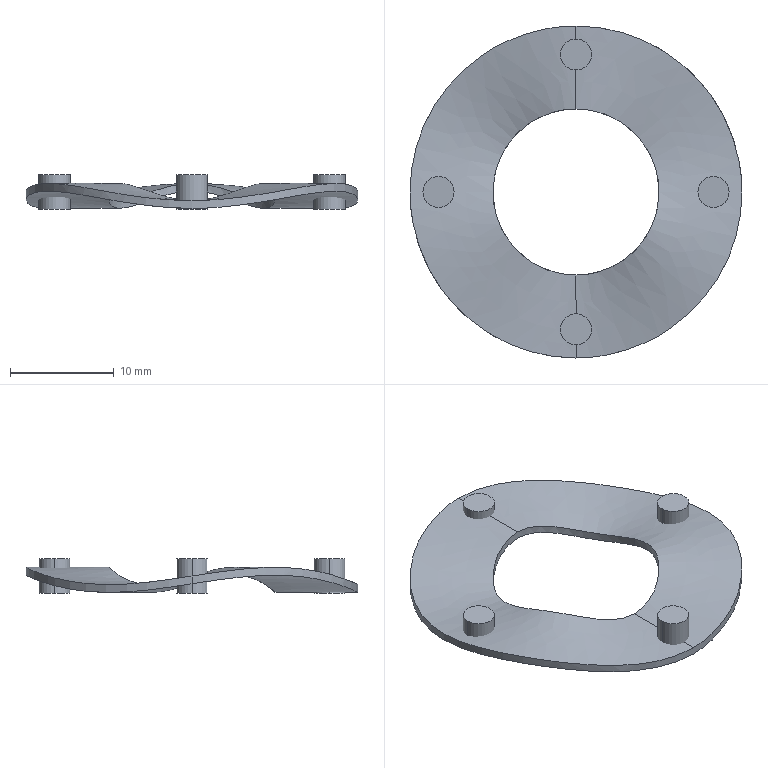Part | NX | 5 solids | 24 faces | box 32 x 32 x 3.35 mm | volume 547.109 mm3 | cylinder 12 | plane 8 | spline 4 | commonest cylinder face diameters 3 x8 16 x2 32 x2
STEP:
#1=CARTESIAN_POINT('',(1.5,13.25,-1.675));
#2=VERTEX_POINT('',#1);
#3=CARTESIAN_POINT('',(-1.5,13.25,-1.675));
#4=VERTEX_POINT('',#3);
#5=CARTESIAN_POINT('',(0.,13.25,-1.675));
#6=DIRECTION('',(0.,0.,1.));
#7=DIRECTION('',(1.,0.,0.));
#8=AXIS2_PLACEMENT_3D('',#5,#6,#7);
#9=CIRCLE('',#8,1.5);
#10=EDGE_CURVE('',#2,#4,#9,.T.);
#11=ORIENTED_EDGE('',*,*,#10,.T.);
#12=CARTESIAN_POINT('',(-1.5,13.25,1.675));
#13=VERTEX_POINT('',#12);
#14=CARTESIAN_POINT('',(-1.5,13.25,-1.675));
#15=DIRECTION('',(0.,0.,1.));
#16=VECTOR('',#15,1.);
#17=LINE('',#14,#16);
#18=EDGE_CURVE('',#4,#13,#17,.T.);
#19=ORIENTED_EDGE('',*,*,#18,.T.);
#20=CARTESIAN_POINT('',(1.5,13.25,1.675));
#21=VERTEX_POINT('',#20);
#22=CARTESIAN_POINT('',(0.,13.25,1.675));
#23=DIRECTION('',(0.,0.,-1.));
#24=DIRECTION('',(1.,0.,0.));
#25=AXIS2_PLACEMENT_3D('',#22,#23,#24);
#26=CIRCLE('',#25,1.5);
#27=EDGE_CURVE('',#13,#21,#26,.T.);
#28=ORIENTED_EDGE('',*,*,#27,.T.);
#29=CARTESIAN_POINT('',(1.5,13.25,-1.675));
#30=DIRECTION('',(0.,0.,1.));
#31=VECTOR('',#30,1.);
#32=LINE('',#29,#31);
#33=EDGE_CURVE('',#2,#21,#32,.T.);
#34=ORIENTED_EDGE('',*,*,#33,.F.);
#35=EDGE_LOOP('',(#11,#19,#28,#34));
#36=FACE_OUTER_BOUND('',#35,.T.);
#37=CARTESIAN_POINT('',(0.,13.25,-1.675));
#38=DIRECTION('',(0.,0.,1.));
#39=DIRECTION('',(1.,0.,0.));
#40=AXIS2_PLACEMENT_3D('',#37,#38,#39);
#41=CYLINDRICAL_SURFACE('',#40,1.5);
#42=ADVANCED_FACE('',(#36),#41,.T.);
#43=ORIENTED_EDGE('',*,*,#18,.F.);
#44=CARTESIAN_POINT('',(0.,13.25,-1.675));
#45=DIRECTION('',(0.,0.,1.));
#46=DIRECTION('',(1.,0.,0.));
#47=AXIS2_PLACEMENT_3D('',#44,#45,#46);
#48=CIRCLE('',#47,1.5);
#49=EDGE_CURVE('',#4,#2,#48,.T.);
#50=ORIENTED_EDGE('',*,*,#49,.T.);
#51=ORIENTED_EDGE('',*,*,#33,.T.);
#52=CARTESIAN_POINT('',(0.,13.25,1.675));
#53=DIRECTION('',(0.,0.,-1.));
#54=DIRECTION('',(1.,0.,0.));
#55=AXIS2_PLACEMENT_3D('',#52,#53,#54);
#56=CIRCLE('',#55,1.5);
#57=EDGE_CURVE('',#21,#13,#56,.T.);
#58=ORIENTED_EDGE('',*,*,#57,.T.);
#59=EDGE_LOOP('',(#43,#50,#51,#58));
#60=FACE_OUTER_BOUND('',#59,.T.);
#61=CARTESIAN_POINT('',(0.,13.25,-1.675));
#62=DIRECTION('',(0.,0.,1.));
#63=DIRECTION('',(1.,0.,0.));
#64=AXIS2_PLACEMENT_3D('',#61,#62,#63);
#65=CYLINDRICAL_SURFACE('',#64,1.5);
#66=ADVANCED_FACE('',(#60),#65,.T.);
#67=ORIENTED_EDGE('',*,*,#10,.F.);
#68=ORIENTED_EDGE('',*,*,#49,.F.);
#69=EDGE_LOOP('',(#67,#68));
#70=FACE_OUTER_BOUND('',#69,.T.);
#71=CARTESIAN_POINT('',(0.,0.,-1.675));
#72=DIRECTION('',(0.,0.,1.));
#73=DIRECTION('',(1.,0.,0.));
#74=AXIS2_PLACEMENT_3D('',#71,#72,#73);
#75=PLANE('',#74);
#76=ADVANCED_FACE('',(#70),#75,.F.);
#77=ORIENTED_EDGE('',*,*,#57,.F.);
#78=ORIENTED_EDGE('',*,*,#27,.F.);
#79=EDGE_LOOP('',(#77,#78));
#80=FACE_OUTER_BOUND('',#79,.T.);
#81=CARTESIAN_POINT('',(0.,0.,1.675));
#82=DIRECTION('',(0.,0.,1.));
#83=DIRECTION('',(1.,0.,0.));
#84=AXIS2_PLACEMENT_3D('',#81,#82,#83);
#85=PLANE('',#84);
#86=ADVANCED_FACE('',(#80),#85,.T.);
#87=CLOSED_SHELL('',(#42,#66,#76,#86));
#88=MANIFOLD_SOLID_BREP('',#87);
#89=CARTESIAN_POINT('',(14.75,0.,-1.675));
#90=VERTEX_POINT('',#89);
#91=CARTESIAN_POINT('',(11.75,0.,-1.675));
#92=VERTEX_POINT('',#91);
#93=CARTESIAN_POINT('',(13.25,0.,-1.675));
#94=DIRECTION('',(0.,0.,1.));
#95=DIRECTION('',(1.,0.,0.));
#96=AXIS2_PLACEMENT_3D('',#93,#94,#95);
#97=CIRCLE('',#96,1.5);
#98=EDGE_CURVE('',#90,#92,#97,.T.);
#99=ORIENTED_EDGE('',*,*,#98,.T.);
#100=CARTESIAN_POINT('',(11.75,0.,1.675));
#101=VERTEX_POINT('',#100);
#102=CARTESIAN_POINT('',(11.75,0.,-1.675));
#103=DIRECTION('',(0.,0.,1.));
#104=VECTOR('',#103,1.);
#105=LINE('',#102,#104);
#106=EDGE_CURVE('',#92,#101,#105,.T.);
#107=ORIENTED_EDGE('',*,*,#106,.T.);
#108=CARTESIAN_POINT('',(14.75,0.,1.675));
#109=VERTEX_POINT('',#108);
#110=CARTESIAN_POINT('',(13.25,0.,1.675));
#111=DIRECTION('',(0.,0.,-1.));
#112=DIRECTION('',(1.,0.,0.));
#113=AXIS2_PLACEMENT_3D('',#110,#111,#112);
#114=CIRCLE('',#113,1.5);
#115=EDGE_CURVE('',#101,#109,#114,.T.);
#116=ORIENTED_EDGE('',*,*,#115,.T.);
#117=CARTESIAN_POINT('',(14.75,0.,-1.675));
#118=DIRECTION('',(0.,0.,1.));
#119=VECTOR('',#118,1.);
#120=LINE('',#117,#119);
#121=EDGE_CURVE('',#90,#109,#120,.T.);
#122=ORIENTED_EDGE('',*,*,#121,.F.);
#123=EDGE_LOOP('',(#99,#107,#116,#122));
#124=FACE_OUTER_BOUND('',#123,.T.);
#125=CARTESIAN_POINT('',(13.25,0.,-1.675));
#126=DIRECTION('',(0.,0.,1.));
#127=DIRECTION('',(1.,0.,0.));
#128=AXIS2_PLACEMENT_3D('',#125,#126,#127);
#129=CYLINDRICAL_SURFACE('',#128,1.5);
#130=ADVANCED_FACE('',(#124),#129,.T.);
#131=ORIENTED_EDGE('',*,*,#106,.F.);
#132=CARTESIAN_POINT('',(13.25,0.,-1.675));
#133=DIRECTION('',(0.,0.,1.));
#134=DIRECTION('',(1.,0.,0.));
#135=AXIS2_PLACEMENT_3D('',#132,#133,#134);
#136=CIRCLE('',#135,1.5);
#137=EDGE_CURVE('',#92,#90,#136,.T.);
#138=ORIENTED_EDGE('',*,*,#137,.T.);
#139=ORIENTED_EDGE('',*,*,#121,.T.);
#140=CARTESIAN_POINT('',(13.25,0.,1.675));
#141=DIRECTION('',(0.,0.,-1.));
#142=DIRECTION('',(1.,0.,0.));
#143=AXIS2_PLACEMENT_3D('',#140,#141,#142);
#144=CIRCLE('',#143,1.5);
#145=EDGE_CURVE('',#109,#101,#144,.T.);
#146=ORIENTED_EDGE('',*,*,#145,.T.);
#147=EDGE_LOOP('',(#131,#138,#139,#146));
#148=FACE_OUTER_BOUND('',#147,.T.);
#149=CARTESIAN_POINT('',(13.25,0.,-1.675));
#150=DIRECTION('',(0.,0.,1.));
#151=DIRECTION('',(1.,0.,0.));
#152=AXIS2_PLACEMENT_3D('',#149,#150,#151);
#153=CYLINDRICAL_SURFACE('',#152,1.5);
#154=ADVANCED_FACE('',(#148),#153,.T.);
#155=ORIENTED_EDGE('',*,*,#98,.F.);
#156=ORIENTED_EDGE('',*,*,#137,.F.);
#157=EDGE_LOOP('',(#155,#156));
#158=FACE_OUTER_BOUND('',#157,.T.);
#159=CARTESIAN_POINT('',(0.,0.,-1.675));
#160=DIRECTION('',(0.,0.,1.));
#161=DIRECTION('',(1.,0.,0.));
#162=AXIS2_PLACEMENT_3D('',#159,#160,#161);
#163=PLANE('',#162);
#164=ADVANCED_FACE('',(#158),#163,.F.);
#165=ORIENTED_EDGE('',*,*,#145,.F.);
#166=ORIENTED_EDGE('',*,*,#115,.F.);
#167=EDGE_LOOP('',(#165,#166));
#168=FACE_OUTER_BOUND('',#167,.T.);
#169=CARTESIAN_POINT('',(0.,0.,1.675));
#170=DIRECTION('',(0.,0.,1.));
#171=DIRECTION('',(1.,0.,0.));
#172=AXIS2_PLACEMENT_3D('',#169,#170,#171);
#173=PLANE('',#172);
#174=ADVANCED_FACE('',(#168),#173,.T.);
#175=CLOSED_SHELL('',(#130,#154,#164,#174));
#176=MANIFOLD_SOLID_BREP('',#175);
#177=CARTESIAN_POINT('',(-11.75,0.,-1.675));
#178=VERTEX_POINT('',#177);
#179=CARTESIAN_POINT('',(-14.75,0.,-1.675));
#180=VERTEX_POINT('',#179);
#181=CARTESIAN_POINT('',(-13.25,0.,-1.675));
#182=DIRECTION('',(0.,0.,1.));
#183=DIRECTION('',(1.,0.,0.));
#184=AXIS2_PLACEMENT_3D('',#181,#182,#183);
#185=CIRCLE('',#184,1.5);
#186=EDGE_CURVE('',#178,#180,#185,.T.);
#187=ORIENTED_EDGE('',*,*,#186,.T.);
#188=CARTESIAN_POINT('',(-14.75,0.,1.675));
#189=VERTEX_POINT('',#188);
#190=CARTESIAN_POINT('',(-14.75,0.,-1.675));
#191=DIRECTION('',(0.,0.,1.));
#192=VECTOR('',#191,1.);
#193=LINE('',#190,#192);
#194=EDGE_CURVE('',#180,#189,#193,.T.);
#195=ORIENTED_EDGE('',*,*,#194,.T.);
#196=CARTESIAN_POINT('',(-11.75,0.,1.675));
#197=VERTEX_POINT('',#196);
#198=CARTESIAN_POINT('',(-13.25,0.,1.675));
#199=DIRECTION('',(0.,0.,-1.));
#200=DIRECTION('',(1.,0.,0.));
#201=AXIS2_PLACEMENT_3D('',#198,#199,#200);
#202=CIRCLE('',#201,1.5);
#203=EDGE_CURVE('',#189,#197,#202,.T.);
#204=ORIENTED_EDGE('',*,*,#203,.T.);
#205=CARTESIAN_POINT('',(-11.75,0.,-1.675));
#206=DIRECTION('',(0.,0.,1.));
#207=VECTOR('',#206,1.);
#208=LINE('',#205,#207);
#209=EDGE_CURVE('',#178,#197,#208,.T.);
#210=ORIENTED_EDGE('',*,*,#209,.F.);
#211=EDGE_LOOP('',(#187,#195,#204,#210));
#212=FACE_OUTER_BOUND('',#211,.T.);
#213=CARTESIAN_POINT('',(-13.25,0.,-1.675));
#214=DIRECTION('',(0.,0.,1.));
#215=DIRECTION('',(1.,0.,0.));
#216=AXIS2_PLACEMENT_3D('',#213,#214,#215);
#217=CYLINDRICAL_SURFACE('',#216,1.5);
#218=ADVANCED_FACE('',(#212),#217,.T.);
#219=ORIENTED_EDGE('',*,*,#194,.F.);
#220=CARTESIAN_POINT('',(-13.25,0.,-1.675));
#221=DIRECTION('',(0.,0.,1.));
#222=DIRECTION('',(1.,0.,0.));
#223=AXIS2_PLACEMENT_3D('',#220,#221,#222);
#224=CIRCLE('',#223,1.5);
#225=EDGE_CURVE('',#180,#178,#224,.T.);
#226=ORIENTED_EDGE('',*,*,#225,.T.);
#227=ORIENTED_EDGE('',*,*,#209,.T.);
#228=CARTESIAN_POINT('',(-13.25,0.,1.675));
#229=DIRECTION('',(0.,0.,-1.));
#230=DIRECTION('',(1.,0.,0.));
#231=AXIS2_PLACEMENT_3D('',#228,#229,#230);
#232=CIRCLE('',#231,1.5);
#233=EDGE_CURVE('',#197,#189,#232,.T.);
#234=ORIENTED_EDGE('',*,*,#233,.T.);
#235=EDGE_LOOP('',(#219,#226,#227,#234));
#236=FACE_OUTER_BOUND('',#235,.T.);
#237=CARTESIAN_POINT('',(-13.25,0.,-1.675));
#238=DIRECTION('',(0.,0.,1.));
#239=DIRECTION('',(1.,0.,0.));
#240=AXIS2_PLACEMENT_3D('',#237,#238,#239);
#241=CYLINDRICAL_SURFACE('',#240,1.5);
#242=ADVANCED_FACE('',(#236),#241,.T.);
#243=ORIENTED_EDGE('',*,*,#186,.F.);
#244=ORIENTED_EDGE('',*,*,#225,.F.);
#245=EDGE_LOOP('',(#243,#244));
#246=FACE_OUTER_BOUND('',#245,.T.);
#247=CARTESIAN_POINT('',(0.,0.,-1.675));
#248=DIRECTION('',(0.,0.,1.));
#249=DIRECTION('',(1.,0.,0.));
#250=AXIS2_PLACEMENT_3D('',#247,#248,#249);
#251=PLANE('',#250);
#252=ADVANCED_FACE('',(#246),#251,.F.);
#253=ORIENTED_EDGE('',*,*,#233,.F.);
#254=ORIENTED_EDGE('',*,*,#203,.F.);
#255=EDGE_LOOP('',(#253,#254));
#256=FACE_OUTER_BOUND('',#255,.T.);
#257=CARTESIAN_POINT('',(0.,0.,1.675));
#258=DIRECTION('',(0.,0.,1.));
#259=DIRECTION('',(1.,0.,0.));
#260=AXIS2_PLACEMENT_3D('',#257,#258,#259);
#261=PLANE('',#260);
#262=ADVANCED_FACE('',(#256),#261,.T.);
#263=CLOSED_SHELL('',(#218,#242,#252,#262));
#264=MANIFOLD_SOLID_BREP('',#263);
#265=CARTESIAN_POINT('',(-16.,0.,-0.75));
#266=VERTEX_POINT('',#265);
#267=CARTESIAN_POINT('',(0.,16.,0.08));
#268=VERTEX_POINT('',#267);
#269=CARTESIAN_POINT('',(-16.,0.,-0.75));
#270=CARTESIAN_POINT('',(-16.,2.1,-1.077));
#271=CARTESIAN_POINT('',(-15.59,4.168,-1.39));
#272=CARTESIAN_POINT('',(-13.983,8.056,-1.642));
#273=CARTESIAN_POINT('',(-12.787,9.841,-1.566));
#274=CARTESIAN_POINT('',(-8.355,14.271,-0.876));
#275=CARTESIAN_POINT('',(-4.255,16.,0.08));
#276=CARTESIAN_POINT('',(0.,16.,0.08));
#277=B_SPLINE_CURVE_WITH_KNOTS('',3,(#269,#270,#271,#272,#273,#274,#275,#276),.UNSPECIFIED.,.F.,.F.,(4,2,2,4),(0.,0.25,0.5,1.),.UNSPECIFIED.);
#278=EDGE_CURVE('',#266,#268,#277,.T.);
#279=ORIENTED_EDGE('',*,*,#278,.F.);
#280=CARTESIAN_POINT('',(-16.,0.,0.));
#281=VERTEX_POINT('',#280);
#282=CARTESIAN_POINT('',(-16.,0.,0.));
#283=DIRECTION('',(0.,0.,1.));
#284=VECTOR('',#283,1.);
#285=LINE('',#282,#284);
#286=EDGE_CURVE('',#266,#281,#285,.T.);
#287=ORIENTED_EDGE('',*,*,#286,.T.);
#288=CARTESIAN_POINT('',(0.,16.,0.83));
#289=VERTEX_POINT('',#288);
#290=CARTESIAN_POINT('',(-16.,0.,0.));
#291=CARTESIAN_POINT('',(-16.,2.1,-0.3267));
#292=CARTESIAN_POINT('',(-15.59,4.168,-0.6399));
#293=CARTESIAN_POINT('',(-13.983,8.056,-0.8922));
#294=CARTESIAN_POINT('',(-12.787,9.841,-0.8164));
#295=CARTESIAN_POINT('',(-8.355,14.271,-0.126));
#296=CARTESIAN_POINT('',(-4.255,16.,0.83));
#297=CARTESIAN_POINT('',(0.,16.,0.83));
#298=B_SPLINE_CURVE_WITH_KNOTS('',3,(#290,#291,#292,#293,#294,#295,#296,#297),.UNSPECIFIED.,.F.,.F.,(4,2,2,4),(0.,0.25,0.5,1.),.UNSPECIFIED.);
#299=EDGE_CURVE('',#281,#289,#298,.T.);
#300=ORIENTED_EDGE('',*,*,#299,.T.);
#301=CARTESIAN_POINT('',(16.,0.,0.));
#302=VERTEX_POINT('',#301);
#303=CARTESIAN_POINT('',(0.,16.,0.83));
#304=CARTESIAN_POINT('',(2.127,16.,0.83));
#305=CARTESIAN_POINT('',(4.213,15.576,0.6153));
#306=CARTESIAN_POINT('',(8.062,13.977,0.01546));
#307=CARTESIAN_POINT('',(9.83,12.795,-0.3554));
#308=CARTESIAN_POINT('',(12.775,9.856,-0.8147));
#309=CARTESIAN_POINT('',(13.98,8.058,-0.8917));
#310=CARTESIAN_POINT('',(15.583,4.189,-0.642));
#311=CARTESIAN_POINT('',(16.,2.1,-0.3268));
#312=CARTESIAN_POINT('',(16.,0.,0.));
#313=B_SPLINE_CURVE_WITH_KNOTS('',3,(#303,#304,#305,#306,#307,#308,#309,#310,#311,#312),.UNSPECIFIED.,.F.,.F.,(4,2,2,2,4),(0.,0.25,0.5,0.75,1.),.UNSPECIFIED.);
#314=EDGE_CURVE('',#289,#302,#313,.T.);
#315=ORIENTED_EDGE('',*,*,#314,.T.);
#316=CARTESIAN_POINT('',(16.,0.,-0.75));
#317=VERTEX_POINT('',#316);
#318=CARTESIAN_POINT('',(16.,0.,0.));
#319=DIRECTION('',(0.,0.,1.));
#320=VECTOR('',#319,1.);
#321=LINE('',#318,#320);
#322=EDGE_CURVE('',#317,#302,#321,.T.);
#323=ORIENTED_EDGE('',*,*,#322,.F.);
#324=CARTESIAN_POINT('',(0.,16.,0.08));
#325=CARTESIAN_POINT('',(4.254,16.,0.08));
#326=CARTESIAN_POINT('',(8.359,14.265,-0.8766));
#327=CARTESIAN_POINT('',(12.782,9.847,-1.566));
#328=CARTESIAN_POINT('',(13.982,8.057,-1.642));
#329=CARTESIAN_POINT('',(15.589,4.172,-1.39));
#330=CARTESIAN_POINT('',(16.,2.1,-1.077));
#331=CARTESIAN_POINT('',(16.,0.,-0.75));
#332=B_SPLINE_CURVE_WITH_KNOTS('',3,(#324,#325,#326,#327,#328,#329,#330,#331),.UNSPECIFIED.,.F.,.F.,(4,2,2,4),(0.,0.5,0.75,1.),.UNSPECIFIED.);
#333=EDGE_CURVE('',#268,#317,#332,.T.);
#334=ORIENTED_EDGE('',*,*,#333,.F.);
#335=EDGE_LOOP('',(#279,#287,#300,#315,#323,#334));
#336=FACE_OUTER_BOUND('',#335,.T.);
#337=CARTESIAN_POINT('',(0.,0.,0.));
#338=DIRECTION('',(0.,0.,1.));
#339=DIRECTION('',(1.,0.,0.));
#340=AXIS2_PLACEMENT_3D('',#337,#338,#339);
#341=CYLINDRICAL_SURFACE('',#340,16.);
#342=ADVANCED_FACE('',(#336),#341,.T.);
#343=CARTESIAN_POINT('',(-8.,0.,-0.75));
#344=VERTEX_POINT('',#343);
#345=CARTESIAN_POINT('',(0.,-8.,-1.58));
#346=VERTEX_POINT('',#345);
#347=CARTESIAN_POINT('',(-8.,0.,-0.75));
#348=CARTESIAN_POINT('',(-8.,-1.03,-0.4294));
#349=CARTESIAN_POINT('',(-7.802,-2.061,-0.1147));
#350=CARTESIAN_POINT('',(-6.996,-4.022,0.1431));
#351=CARTESIAN_POINT('',(-6.383,-4.937,0.06444));
#352=CARTESIAN_POINT('',(-4.14,-7.162,-0.6387));
#353=CARTESIAN_POINT('',(-2.165,-8.,-1.58));
#354=CARTESIAN_POINT('',(0.,-8.,-1.58));
#355=B_SPLINE_CURVE_WITH_KNOTS('',3,(#347,#348,#349,#350,#351,#352,#353,#354),.UNSPECIFIED.,.F.,.F.,(4,2,2,4),(0.,0.25,0.5,1.),.UNSPECIFIED.);
#356=EDGE_CURVE('',#344,#346,#355,.T.);
#357=ORIENTED_EDGE('',*,*,#356,.F.);
#358=CARTESIAN_POINT('',(-8.,0.,0.));
#359=VERTEX_POINT('',#358);
#360=CARTESIAN_POINT('',(-8.,0.,0.));
#361=DIRECTION('',(0.,0.,1.));
#362=VECTOR('',#361,1.);
#363=LINE('',#360,#362);
#364=EDGE_CURVE('',#344,#359,#363,.T.);
#365=ORIENTED_EDGE('',*,*,#364,.T.);
#366=CARTESIAN_POINT('',(0.,-8.,-0.83));
#367=VERTEX_POINT('',#366);
#368=CARTESIAN_POINT('',(0.,-8.,-0.83));
#369=CARTESIAN_POINT('',(-2.167,-8.,-0.83));
#370=CARTESIAN_POINT('',(-4.151,-7.146,0.113));
#371=CARTESIAN_POINT('',(-6.361,-4.961,0.8085));
#372=CARTESIAN_POINT('',(-6.983,-4.05,0.8951));
#373=CARTESIAN_POINT('',(-7.804,-2.061,0.6369));
#374=CARTESIAN_POINT('',(-8.,-1.033,0.3215));
#375=CARTESIAN_POINT('',(-8.,0.,0.));
#376=B_SPLINE_CURVE_WITH_KNOTS('',3,(#368,#369,#370,#371,#372,#373,#374,#375),.UNSPECIFIED.,.F.,.F.,(4,2,2,4),(0.,0.5,0.75,1.),.UNSPECIFIED.);
#377=EDGE_CURVE('',#367,#359,#376,.T.);
#378=ORIENTED_EDGE('',*,*,#377,.F.);
#379=CARTESIAN_POINT('',(8.,0.,0.));
#380=VERTEX_POINT('',#379);
#381=CARTESIAN_POINT('',(8.,0.,0.));
#382=CARTESIAN_POINT('',(8.,-1.03,0.3206));
#383=CARTESIAN_POINT('',(7.802,-2.061,0.6352));
#384=CARTESIAN_POINT('',(6.996,-4.022,0.8931));
#385=CARTESIAN_POINT('',(6.382,-4.937,0.8144));
#386=CARTESIAN_POINT('',(4.141,-7.161,0.1115));
#387=CARTESIAN_POINT('',(2.165,-8.,-0.83));
#388=CARTESIAN_POINT('',(0.,-8.,-0.83));
#389=B_SPLINE_CURVE_WITH_KNOTS('',3,(#381,#382,#383,#384,#385,#386,#387,#388),.UNSPECIFIED.,.F.,.F.,(4,2,2,4),(0.,0.25,0.5,1.),.UNSPECIFIED.);
#390=EDGE_CURVE('',#380,#367,#389,.T.);
#391=ORIENTED_EDGE('',*,*,#390,.F.);
#392=CARTESIAN_POINT('',(8.,0.,-0.75));
#393=VERTEX_POINT('',#392);
#394=CARTESIAN_POINT('',(8.,0.,0.));
#395=DIRECTION('',(0.,0.,1.));
#396=VECTOR('',#395,1.);
#397=LINE('',#394,#396);
#398=EDGE_CURVE('',#393,#380,#397,.T.);
#399=ORIENTED_EDGE('',*,*,#398,.F.);
#400=CARTESIAN_POINT('',(0.,-8.,-1.58));
#401=CARTESIAN_POINT('',(2.167,-8.,-1.58));
#402=CARTESIAN_POINT('',(4.151,-7.146,-0.637));
#403=CARTESIAN_POINT('',(6.361,-4.961,0.0585));
#404=CARTESIAN_POINT('',(6.983,-4.05,0.1451));
#405=CARTESIAN_POINT('',(7.804,-2.061,-0.1131));
#406=CARTESIAN_POINT('',(8.,-1.033,-0.4285));
#407=CARTESIAN_POINT('',(8.,0.,-0.75));
#408=B_SPLINE_CURVE_WITH_KNOTS('',3,(#400,#401,#402,#403,#404,#405,#406,#407),.UNSPECIFIED.,.F.,.F.,(4,2,2,4),(0.,0.5,0.75,1.),.UNSPECIFIED.);
#409=EDGE_CURVE('',#346,#393,#408,.T.);
#410=ORIENTED_EDGE('',*,*,#409,.F.);
#411=EDGE_LOOP('',(#357,#365,#378,#391,#399,#410));
#412=FACE_OUTER_BOUND('',#411,.T.);
#413=CARTESIAN_POINT('',(0.,0.,0.));
#414=DIRECTION('',(0.,0.,1.));
#415=DIRECTION('',(1.,0.,0.));
#416=AXIS2_PLACEMENT_3D('',#413,#414,#415);
#417=CYLINDRICAL_SURFACE('',#416,8.);
#418=ADVANCED_FACE('',(#412),#417,.F.);
#419=ORIENTED_EDGE('',*,*,#333,.T.);
#420=CARTESIAN_POINT('',(0.,-16.,-1.58));
#421=VERTEX_POINT('',#420);
#422=CARTESIAN_POINT('',(16.,0.,-0.75));
#423=CARTESIAN_POINT('',(16.,-2.1,-0.4233));
#424=CARTESIAN_POINT('',(15.59,-4.168,-0.1101));
#425=CARTESIAN_POINT('',(13.983,-8.056,0.1422));
#426=CARTESIAN_POINT('',(12.787,-9.841,0.06634));
#427=CARTESIAN_POINT('',(8.355,-14.271,-0.624));
#428=CARTESIAN_POINT('',(4.255,-16.,-1.58));
#429=CARTESIAN_POINT('',(0.,-16.,-1.58));
#430=B_SPLINE_CURVE_WITH_KNOTS('',3,(#422,#423,#424,#425,#426,#427,#428,#429),.UNSPECIFIED.,.F.,.F.,(4,2,2,4),(0.,0.25,0.5,1.),.UNSPECIFIED.);
#431=EDGE_CURVE('',#317,#421,#430,.T.);
#432=ORIENTED_EDGE('',*,*,#431,.T.);
#433=CARTESIAN_POINT('',(0.,-12.,-1.58));
#434=DIRECTION('',(0.,1.,0.));
#435=VECTOR('',#434,1.);
#436=LINE('',#433,#435);
#437=EDGE_CURVE('',#421,#346,#436,.T.);
#438=ORIENTED_EDGE('',*,*,#437,.T.);
#439=ORIENTED_EDGE('',*,*,#409,.T.);
#440=CARTESIAN_POINT('',(0.,8.,0.08));
#441=VERTEX_POINT('',#440);
#442=CARTESIAN_POINT('',(8.,0.,-0.75));
#443=CARTESIAN_POINT('',(8.,1.03,-1.071));
#444=CARTESIAN_POINT('',(7.802,2.061,-1.385));
#445=CARTESIAN_POINT('',(6.996,4.022,-1.643));
#446=CARTESIAN_POINT('',(6.383,4.937,-1.564));
#447=CARTESIAN_POINT('',(4.14,7.162,-0.8613));
#448=CARTESIAN_POINT('',(2.165,8.,0.08));
#449=CARTESIAN_POINT('',(0.,8.,0.08));
#450=B_SPLINE_CURVE_WITH_KNOTS('',3,(#442,#443,#444,#445,#446,#447,#448,#449),.UNSPECIFIED.,.F.,.F.,(4,2,2,4),(0.,0.25,0.5,1.),.UNSPECIFIED.);
#451=EDGE_CURVE('',#393,#441,#450,.T.);
#452=ORIENTED_EDGE('',*,*,#451,.T.);
#453=CARTESIAN_POINT('',(0.,12.,0.08));
#454=DIRECTION('',(0.,1.,0.));
#455=VECTOR('',#454,1.);
#456=LINE('',#453,#455);
#457=EDGE_CURVE('',#441,#268,#456,.T.);
#458=ORIENTED_EDGE('',*,*,#457,.T.);
#459=EDGE_LOOP('',(#419,#432,#438,#439,#452,#458));
#460=FACE_OUTER_BOUND('',#459,.T.);
#461=CARTESIAN_POINT('',(-1.015,-16.128,-1.565));
#462=CARTESIAN_POINT('',(0.09079,-16.198,-1.598));
#463=CARTESIAN_POINT('',(1.976,-16.122,-1.56));
#464=CARTESIAN_POINT('',(4.568,-15.558,-1.31));
#465=CARTESIAN_POINT('',(6.736,-14.75,-0.9911));
#466=CARTESIAN_POINT('',(8.766,-13.641,-0.6282));
#467=CARTESIAN_POINT('',(10.619,-12.254,-0.2873));
#468=CARTESIAN_POINT('',(12.254,-10.619,-0.03007));
#469=CARTESIAN_POINT('',(13.641,-8.766,0.09707));
#470=CARTESIAN_POINT('',(14.75,-6.736,0.07111));
#471=CARTESIAN_POINT('',(15.558,-4.568,-0.1032));
#472=CARTESIAN_POINT('',(16.05,-2.308,-0.3945));
#473=CARTESIAN_POINT('',(16.215,0.,-0.75));
#474=CARTESIAN_POINT('',(16.05,2.308,-1.106));
#475=CARTESIAN_POINT('',(15.558,4.568,-1.397));
#476=CARTESIAN_POINT('',(14.75,6.736,-1.571));
#477=CARTESIAN_POINT('',(13.641,8.766,-1.597));
#478=CARTESIAN_POINT('',(12.254,10.619,-1.47));
#479=CARTESIAN_POINT('',(10.619,12.254,-1.213));
#480=CARTESIAN_POINT('',(8.766,13.641,-0.8718));
#481=CARTESIAN_POINT('',(6.736,14.75,-0.5089));
#482=CARTESIAN_POINT('',(4.568,15.558,-0.1896));
#483=CARTESIAN_POINT('',(1.976,16.122,0.06042));
#484=CARTESIAN_POINT('',(0.09079,16.198,0.09815));
#485=CARTESIAN_POINT('',(-1.015,16.128,0.06483));
#486=CARTESIAN_POINT('',(-0.8406,-13.36,-1.565));
#487=CARTESIAN_POINT('',(0.07521,-13.418,-1.598));
#488=CARTESIAN_POINT('',(1.637,-13.355,-1.56));
#489=CARTESIAN_POINT('',(3.784,-12.888,-1.31));
#490=CARTESIAN_POINT('',(5.58,-12.218,-0.9911));
#491=CARTESIAN_POINT('',(7.262,-11.3,-0.6282));
#492=CARTESIAN_POINT('',(8.796,-10.151,-0.2873));
#493=CARTESIAN_POINT('',(10.151,-8.796,-0.03007));
#494=CARTESIAN_POINT('',(11.3,-7.262,0.09707));
#495=CARTESIAN_POINT('',(12.218,-5.58,0.07111));
#496=CARTESIAN_POINT('',(12.888,-3.784,-0.1032));
#497=CARTESIAN_POINT('',(13.296,-1.912,-0.3945));
#498=CARTESIAN_POINT('',(13.432,0.,-0.75));
#499=CARTESIAN_POINT('',(13.296,1.912,-1.106));
#500=CARTESIAN_POINT('',(12.888,3.784,-1.397));
#501=CARTESIAN_POINT('',(12.218,5.58,-1.571));
#502=CARTESIAN_POINT('',(11.3,7.262,-1.597));
#503=CARTESIAN_POINT('',(10.151,8.796,-1.47));
#504=CARTESIAN_POINT('',(8.796,10.151,-1.213));
#505=CARTESIAN_POINT('',(7.262,11.3,-0.8718));
#506=CARTESIAN_POINT('',(5.58,12.218,-0.5089));
#507=CARTESIAN_POINT('',(3.784,12.888,-0.1896));
#508=CARTESIAN_POINT('',(1.637,13.355,0.06042));
#509=CARTESIAN_POINT('',(0.07521,13.418,0.09815));
#510=CARTESIAN_POINT('',(-0.8406,13.36,0.06483));
#511=CARTESIAN_POINT('',(-0.6664,-10.592,-1.565));
#512=CARTESIAN_POINT('',(0.05963,-10.638,-1.598));
#513=CARTESIAN_POINT('',(1.298,-10.588,-1.56));
#514=CARTESIAN_POINT('',(3.,-10.218,-1.31));
#515=CARTESIAN_POINT('',(4.424,-9.687,-0.9911));
#516=CARTESIAN_POINT('',(5.758,-8.959,-0.6282));
#517=CARTESIAN_POINT('',(6.974,-8.048,-0.2873));
#518=CARTESIAN_POINT('',(8.048,-6.974,-0.03007));
#519=CARTESIAN_POINT('',(8.959,-5.758,0.09707));
#520=CARTESIAN_POINT('',(9.687,-4.424,0.07111));
#521=CARTESIAN_POINT('',(10.218,-3.,-0.1032));
#522=CARTESIAN_POINT('',(10.541,-1.516,-0.3945));
#523=CARTESIAN_POINT('',(10.649,0.,-0.75));
#524=CARTESIAN_POINT('',(10.541,1.516,-1.106));
#525=CARTESIAN_POINT('',(10.218,3.,-1.397));
#526=CARTESIAN_POINT('',(9.687,4.424,-1.571));
#527=CARTESIAN_POINT('',(8.959,5.758,-1.597));
#528=CARTESIAN_POINT('',(8.048,6.974,-1.47));
#529=CARTESIAN_POINT('',(6.974,8.048,-1.213));
#530=CARTESIAN_POINT('',(5.758,8.959,-0.8718));
#531=CARTESIAN_POINT('',(4.424,9.687,-0.5089));
#532=CARTESIAN_POINT('',(3.,10.218,-0.1896));
#533=CARTESIAN_POINT('',(1.298,10.588,0.06042));
#534=CARTESIAN_POINT('',(0.05963,10.638,0.09815));
#535=CARTESIAN_POINT('',(-0.6664,10.592,0.06483));
#536=CARTESIAN_POINT('',(-0.4923,-7.825,-1.565));
#537=CARTESIAN_POINT('',(0.04405,-7.858,-1.598));
#538=CARTESIAN_POINT('',(0.9587,-7.822,-1.56));
#539=CARTESIAN_POINT('',(2.216,-7.548,-1.31));
#540=CARTESIAN_POINT('',(3.268,-7.156,-0.9911));
#541=CARTESIAN_POINT('',(4.253,-6.618,-0.6282));
#542=CARTESIAN_POINT('',(5.152,-5.945,-0.2873));
#543=CARTESIAN_POINT('',(5.945,-5.152,-0.03007));
#544=CARTESIAN_POINT('',(6.618,-4.253,0.09707));
#545=CARTESIAN_POINT('',(7.156,-3.268,0.07111));
#546=CARTESIAN_POINT('',(7.548,-2.216,-0.1032));
#547=CARTESIAN_POINT('',(7.787,-1.12,-0.3945));
#548=CARTESIAN_POINT('',(7.867,0.,-0.75));
#549=CARTESIAN_POINT('',(7.787,1.12,-1.106));
#550=CARTESIAN_POINT('',(7.548,2.216,-1.397));
#551=CARTESIAN_POINT('',(7.156,3.268,-1.571));
#552=CARTESIAN_POINT('',(6.618,4.253,-1.597));
#553=CARTESIAN_POINT('',(5.945,5.152,-1.47));
#554=CARTESIAN_POINT('',(5.152,5.945,-1.213));
#555=CARTESIAN_POINT('',(4.253,6.618,-0.8718));
#556=CARTESIAN_POINT('',(3.268,7.156,-0.5089));
#557=CARTESIAN_POINT('',(2.216,7.548,-0.1896));
#558=CARTESIAN_POINT('',(0.9587,7.822,0.06042));
#559=CARTESIAN_POINT('',(0.04405,7.858,0.09815));
#560=CARTESIAN_POINT('',(-0.4923,7.825,0.06483));
#561=B_SPLINE_SURFACE_WITH_KNOTS('',3,3,((#461,#462,#463,#464,#465,#466,#467,#468,#469,#470,#471,#472,#473,#474,#475,#476,#477,#478,#479,#480,#481,#482,#483,#484,#485),(#486,#487,#488,#489,#490,#491,#492,#493,#494,#495,#496,#497,#498,#499,#500,#501,#502,#503,#504,#505,#506,#507,#508,#509,#510),(#511,#512,#513,#514,#515,#516,#517,#518,#519,#520,#521,#522,#523,#524,#525,#526,#527,#528,#529,#530,#531,#532,#533,#534,#535),(#536,#537,#538,#539,#540,#541,#542,#543,#544,#545,#546,#547,#548,#549,#550,#551,#552,#553,#554,#555,#556,#557,#558,#559,#560)),.UNSPECIFIED.,.F.,.F.,.F.,(4,4),(4,1,1,1,1,1,1,1,1,1,1,1,1,1,1,1,1,1,1,1,1,1,4),(0.,1.),(0.,0.06294,0.1066,0.1503,0.1941,0.2378,0.2815,0.3252,0.3689,0.4126,0.4563,0.5,0.5437,0.5874,0.6311,0.6748,0.7185,0.7622,0.8059,0.8497,0.8934,0.9371,1.),.UNSPECIFIED.);
#562=ADVANCED_FACE('',(#460),#561,.T.);
#563=CARTESIAN_POINT('',(0.,-16.,-1.58));
#564=CARTESIAN_POINT('',(-4.254,-16.,-1.58));
#565=CARTESIAN_POINT('',(-8.359,-14.265,-0.6234));
#566=CARTESIAN_POINT('',(-12.782,-9.847,0.06558));
#567=CARTESIAN_POINT('',(-13.982,-8.057,0.1422));
#568=CARTESIAN_POINT('',(-15.589,-4.172,-0.1097));
#569=CARTESIAN_POINT('',(-16.,-2.1,-0.4233));
#570=CARTESIAN_POINT('',(-16.,0.,-0.75));
#571=B_SPLINE_CURVE_WITH_KNOTS('',3,(#563,#564,#565,#566,#567,#568,#569,#570),.UNSPECIFIED.,.F.,.F.,(4,2,2,4),(0.,0.5,0.75,1.),.UNSPECIFIED.);
#572=EDGE_CURVE('',#421,#266,#571,.T.);
#573=ORIENTED_EDGE('',*,*,#572,.T.);
#574=ORIENTED_EDGE('',*,*,#278,.T.);
#575=ORIENTED_EDGE('',*,*,#457,.F.);
#576=CARTESIAN_POINT('',(0.,8.,0.08));
#577=CARTESIAN_POINT('',(-2.167,8.,0.08));
#578=CARTESIAN_POINT('',(-4.151,7.146,-0.863));
#579=CARTESIAN_POINT('',(-6.361,4.961,-1.559));
#580=CARTESIAN_POINT('',(-6.983,4.05,-1.645));
#581=CARTESIAN_POINT('',(-7.804,2.061,-1.387));
#582=CARTESIAN_POINT('',(-8.,1.033,-1.071));
#583=CARTESIAN_POINT('',(-8.,0.,-0.75));
#584=B_SPLINE_CURVE_WITH_KNOTS('',3,(#576,#577,#578,#579,#580,#581,#582,#583),.UNSPECIFIED.,.F.,.F.,(4,2,2,4),(0.,0.5,0.75,1.),.UNSPECIFIED.);
#585=EDGE_CURVE('',#441,#344,#584,.T.);
#586=ORIENTED_EDGE('',*,*,#585,.T.);
#587=ORIENTED_EDGE('',*,*,#356,.T.);
#588=ORIENTED_EDGE('',*,*,#437,.F.);
#589=EDGE_LOOP('',(#573,#574,#575,#586,#587,#588));
#590=FACE_OUTER_BOUND('',#589,.T.);
#591=CARTESIAN_POINT('',(1.015,16.128,0.06483));
#592=CARTESIAN_POINT('',(-0.09079,16.198,0.09815));
#593=CARTESIAN_POINT('',(-1.976,16.122,0.06042));
#594=CARTESIAN_POINT('',(-4.568,15.558,-0.1896));
#595=CARTESIAN_POINT('',(-6.736,14.75,-0.5089));
#596=CARTESIAN_POINT('',(-8.766,13.641,-0.8718));
#597=CARTESIAN_POINT('',(-10.619,12.254,-1.213));
#598=CARTESIAN_POINT('',(-12.254,10.619,-1.47));
#599=CARTESIAN_POINT('',(-13.641,8.766,-1.597));
#600=CARTESIAN_POINT('',(-14.75,6.736,-1.571));
#601=CARTESIAN_POINT('',(-15.558,4.568,-1.397));
#602=CARTESIAN_POINT('',(-16.05,2.308,-1.106));
#603=CARTESIAN_POINT('',(-16.215,0.,-0.75));
#604=CARTESIAN_POINT('',(-16.05,-2.308,-0.3945));
#605=CARTESIAN_POINT('',(-15.558,-4.568,-0.1032));
#606=CARTESIAN_POINT('',(-14.75,-6.736,0.07111));
#607=CARTESIAN_POINT('',(-13.641,-8.766,0.09707));
#608=CARTESIAN_POINT('',(-12.254,-10.619,-0.03007));
#609=CARTESIAN_POINT('',(-10.619,-12.254,-0.2873));
#610=CARTESIAN_POINT('',(-8.766,-13.641,-0.6282));
#611=CARTESIAN_POINT('',(-6.736,-14.75,-0.9911));
#612=CARTESIAN_POINT('',(-4.568,-15.558,-1.31));
#613=CARTESIAN_POINT('',(-1.976,-16.122,-1.56));
#614=CARTESIAN_POINT('',(-0.09079,-16.198,-1.598));
#615=CARTESIAN_POINT('',(1.015,-16.128,-1.565));
#616=CARTESIAN_POINT('',(0.8406,13.36,0.06483));
#617=CARTESIAN_POINT('',(-0.07521,13.418,0.09815));
#618=CARTESIAN_POINT('',(-1.637,13.355,0.06042));
#619=CARTESIAN_POINT('',(-3.784,12.888,-0.1896));
#620=CARTESIAN_POINT('',(-5.58,12.218,-0.5089));
#621=CARTESIAN_POINT('',(-7.262,11.3,-0.8718));
#622=CARTESIAN_POINT('',(-8.796,10.151,-1.213));
#623=CARTESIAN_POINT('',(-10.151,8.796,-1.47));
#624=CARTESIAN_POINT('',(-11.3,7.262,-1.597));
#625=CARTESIAN_POINT('',(-12.218,5.58,-1.571));
#626=CARTESIAN_POINT('',(-12.888,3.784,-1.397));
#627=CARTESIAN_POINT('',(-13.296,1.912,-1.106));
#628=CARTESIAN_POINT('',(-13.432,0.,-0.75));
#629=CARTESIAN_POINT('',(-13.296,-1.912,-0.3945));
#630=CARTESIAN_POINT('',(-12.888,-3.784,-0.1032));
#631=CARTESIAN_POINT('',(-12.218,-5.58,0.07111));
#632=CARTESIAN_POINT('',(-11.3,-7.262,0.09707));
#633=CARTESIAN_POINT('',(-10.151,-8.796,-0.03007));
#634=CARTESIAN_POINT('',(-8.796,-10.151,-0.2873));
#635=CARTESIAN_POINT('',(-7.262,-11.3,-0.6282));
#636=CARTESIAN_POINT('',(-5.58,-12.218,-0.9911));
#637=CARTESIAN_POINT('',(-3.784,-12.888,-1.31));
#638=CARTESIAN_POINT('',(-1.637,-13.355,-1.56));
#639=CARTESIAN_POINT('',(-0.07521,-13.418,-1.598));
#640=CARTESIAN_POINT('',(0.8406,-13.36,-1.565));
#641=CARTESIAN_POINT('',(0.6664,10.592,0.06483));
#642=CARTESIAN_POINT('',(-0.05963,10.638,0.09815));
#643=CARTESIAN_POINT('',(-1.298,10.588,0.06042));
#644=CARTESIAN_POINT('',(-3.,10.218,-0.1896));
#645=CARTESIAN_POINT('',(-4.424,9.687,-0.5089));
#646=CARTESIAN_POINT('',(-5.758,8.959,-0.8718));
#647=CARTESIAN_POINT('',(-6.974,8.048,-1.213));
#648=CARTESIAN_POINT('',(-8.048,6.974,-1.47));
#649=CARTESIAN_POINT('',(-8.959,5.758,-1.597));
#650=CARTESIAN_POINT('',(-9.687,4.424,-1.571));
#651=CARTESIAN_POINT('',(-10.218,3.,-1.397));
#652=CARTESIAN_POINT('',(-10.541,1.516,-1.106));
#653=CARTESIAN_POINT('',(-10.649,0.,-0.75));
#654=CARTESIAN_POINT('',(-10.541,-1.516,-0.3945));
#655=CARTESIAN_POINT('',(-10.218,-3.,-0.1032));
#656=CARTESIAN_POINT('',(-9.687,-4.424,0.07111));
#657=CARTESIAN_POINT('',(-8.959,-5.758,0.09707));
#658=CARTESIAN_POINT('',(-8.048,-6.974,-0.03007));
#659=CARTESIAN_POINT('',(-6.974,-8.048,-0.2873));
#660=CARTESIAN_POINT('',(-5.758,-8.959,-0.6282));
#661=CARTESIAN_POINT('',(-4.424,-9.687,-0.9911));
#662=CARTESIAN_POINT('',(-3.,-10.218,-1.31));
#663=CARTESIAN_POINT('',(-1.298,-10.588,-1.56));
#664=CARTESIAN_POINT('',(-0.05963,-10.638,-1.598));
#665=CARTESIAN_POINT('',(0.6664,-10.592,-1.565));
#666=CARTESIAN_POINT('',(0.4923,7.825,0.06483));
#667=CARTESIAN_POINT('',(-0.04405,7.858,0.09815));
#668=CARTESIAN_POINT('',(-0.9587,7.822,0.06042));
#669=CARTESIAN_POINT('',(-2.216,7.548,-0.1896));
#670=CARTESIAN_POINT('',(-3.268,7.156,-0.5089));
#671=CARTESIAN_POINT('',(-4.253,6.618,-0.8718));
#672=CARTESIAN_POINT('',(-5.152,5.945,-1.213));
#673=CARTESIAN_POINT('',(-5.945,5.152,-1.47));
#674=CARTESIAN_POINT('',(-6.618,4.253,-1.597));
#675=CARTESIAN_POINT('',(-7.156,3.268,-1.571));
#676=CARTESIAN_POINT('',(-7.548,2.216,-1.397));
#677=CARTESIAN_POINT('',(-7.787,1.12,-1.106));
#678=CARTESIAN_POINT('',(-7.867,0.,-0.75));
#679=CARTESIAN_POINT('',(-7.787,-1.12,-0.3945));
#680=CARTESIAN_POINT('',(-7.548,-2.216,-0.1032));
#681=CARTESIAN_POINT('',(-7.156,-3.268,0.07111));
#682=CARTESIAN_POINT('',(-6.618,-4.253,0.09707));
#683=CARTESIAN_POINT('',(-5.945,-5.152,-0.03007));
#684=CARTESIAN_POINT('',(-5.152,-5.945,-0.2873));
#685=CARTESIAN_POINT('',(-4.253,-6.618,-0.6282));
#686=CARTESIAN_POINT('',(-3.268,-7.156,-0.9911));
#687=CARTESIAN_POINT('',(-2.216,-7.548,-1.31));
#688=CARTESIAN_POINT('',(-0.9587,-7.822,-1.56));
#689=CARTESIAN_POINT('',(-0.04405,-7.858,-1.598));
#690=CARTESIAN_POINT('',(0.4923,-7.825,-1.565));
#691=B_SPLINE_SURFACE_WITH_KNOTS('',3,3,((#591,#592,#593,#594,#595,#596,#597,#598,#599,#600,#601,#602,#603,#604,#605,#606,#607,#608,#609,#610,#611,#612,#613,#614,#615),(#616,#617,#618,#619,#620,#621,#622,#623,#624,#625,#626,#627,#628,#629,#630,#631,#632,#633,#634,#635,#636,#637,#638,#639,#640),(#641,#642,#643,#644,#645,#646,#647,#648,#649,#650,#651,#652,#653,#654,#655,#656,#657,#658,#659,#660,#661,#662,#663,#664,#665),(#666,#667,#668,#669,#670,#671,#672,#673,#674,#675,#676,#677,#678,#679,#680,#681,#682,#683,#684,#685,#686,#687,#688,#689,#690)),.UNSPECIFIED.,.F.,.F.,.F.,(4,4),(4,1,1,1,1,1,1,1,1,1,1,1,1,1,1,1,1,1,1,1,1,1,4),(0.,1.),(0.,0.06294,0.1066,0.1503,0.1941,0.2378,0.2815,0.3252,0.3689,0.4126,0.4563,0.5,0.5437,0.5874,0.6311,0.6748,0.7185,0.7622,0.8059,0.8497,0.8934,0.9371,1.),.UNSPECIFIED.);
#692=ADVANCED_FACE('',(#590),#691,.T.);
#693=ORIENTED_EDGE('',*,*,#286,.F.);
#694=ORIENTED_EDGE('',*,*,#572,.F.);
#695=ORIENTED_EDGE('',*,*,#431,.F.);
#696=ORIENTED_EDGE('',*,*,#322,.T.);
#697=CARTESIAN_POINT('',(0.,-16.,-0.83));
#698=VERTEX_POINT('',#697);
#699=CARTESIAN_POINT('',(16.,0.,0.));
#700=CARTESIAN_POINT('',(16.,-2.1,0.3267));
#701=CARTESIAN_POINT('',(15.59,-4.168,0.6399));
#702=CARTESIAN_POINT('',(13.983,-8.056,0.8922));
#703=CARTESIAN_POINT('',(12.787,-9.841,0.8164));
#704=CARTESIAN_POINT('',(8.355,-14.271,0.126));
#705=CARTESIAN_POINT('',(4.255,-16.,-0.83));
#706=CARTESIAN_POINT('',(0.,-16.,-0.83));
#707=B_SPLINE_CURVE_WITH_KNOTS('',3,(#699,#700,#701,#702,#703,#704,#705,#706),.UNSPECIFIED.,.F.,.F.,(4,2,2,4),(0.,0.25,0.5,1.),.UNSPECIFIED.);
#708=EDGE_CURVE('',#302,#698,#707,.T.);
#709=ORIENTED_EDGE('',*,*,#708,.T.);
#710=CARTESIAN_POINT('',(0.,-16.,-0.83));
#711=CARTESIAN_POINT('',(-2.127,-16.,-0.83));
#712=CARTESIAN_POINT('',(-4.213,-15.576,-0.6153));
#713=CARTESIAN_POINT('',(-8.062,-13.977,-0.01546));
#714=CARTESIAN_POINT('',(-9.83,-12.795,0.3554));
#715=CARTESIAN_POINT('',(-12.775,-9.856,0.8147));
#716=CARTESIAN_POINT('',(-13.98,-8.058,0.8917));
#717=CARTESIAN_POINT('',(-15.583,-4.189,0.642));
#718=CARTESIAN_POINT('',(-16.,-2.1,0.3268));
#719=CARTESIAN_POINT('',(-16.,0.,0.));
#720=B_SPLINE_CURVE_WITH_KNOTS('',3,(#710,#711,#712,#713,#714,#715,#716,#717,#718,#719),.UNSPECIFIED.,.F.,.F.,(4,2,2,2,4),(0.,0.25,0.5,0.75,1.),.UNSPECIFIED.);
#721=EDGE_CURVE('',#698,#281,#720,.T.);
#722=ORIENTED_EDGE('',*,*,#721,.T.);
#723=EDGE_LOOP('',(#693,#694,#695,#696,#709,#722));
#724=FACE_OUTER_BOUND('',#723,.T.);
#725=CARTESIAN_POINT('',(0.,0.,0.));
#726=DIRECTION('',(0.,0.,1.));
#727=DIRECTION('',(1.,0.,0.));
#728=AXIS2_PLACEMENT_3D('',#725,#726,#727);
#729=CYLINDRICAL_SURFACE('',#728,16.);
#730=ADVANCED_FACE('',(#724),#729,.T.);
#731=ORIENTED_EDGE('',*,*,#364,.F.);
#732=ORIENTED_EDGE('',*,*,#585,.F.);
#733=ORIENTED_EDGE('',*,*,#451,.F.);
#734=ORIENTED_EDGE('',*,*,#398,.T.);
#735=CARTESIAN_POINT('',(0.,8.,0.83));
#736=VERTEX_POINT('',#735);
#737=CARTESIAN_POINT('',(0.,8.,0.83));
#738=CARTESIAN_POINT('',(2.167,8.,0.83));
#739=CARTESIAN_POINT('',(4.151,7.146,-0.113));
#740=CARTESIAN_POINT('',(6.361,4.961,-0.8085));
#741=CARTESIAN_POINT('',(6.983,4.05,-0.8951));
#742=CARTESIAN_POINT('',(7.804,2.061,-0.6369));
#743=CARTESIAN_POINT('',(8.,1.033,-0.3215));
#744=CARTESIAN_POINT('',(8.,0.,0.));
#745=B_SPLINE_CURVE_WITH_KNOTS('',3,(#737,#738,#739,#740,#741,#742,#743,#744),.UNSPECIFIED.,.F.,.F.,(4,2,2,4),(0.,0.5,0.75,1.),.UNSPECIFIED.);
#746=EDGE_CURVE('',#736,#380,#745,.T.);
#747=ORIENTED_EDGE('',*,*,#746,.F.);
#748=CARTESIAN_POINT('',(-8.,0.,0.));
#749=CARTESIAN_POINT('',(-8.,1.03,-0.3206));
#750=CARTESIAN_POINT('',(-7.802,2.061,-0.6352));
#751=CARTESIAN_POINT('',(-6.996,4.022,-0.8931));
#752=CARTESIAN_POINT('',(-6.382,4.937,-0.8144));
#753=CARTESIAN_POINT('',(-4.141,7.161,-0.1115));
#754=CARTESIAN_POINT('',(-2.165,8.,0.83));
#755=CARTESIAN_POINT('',(0.,8.,0.83));
#756=B_SPLINE_CURVE_WITH_KNOTS('',3,(#748,#749,#750,#751,#752,#753,#754,#755),.UNSPECIFIED.,.F.,.F.,(4,2,2,4),(0.,0.25,0.5,1.),.UNSPECIFIED.);
#757=EDGE_CURVE('',#359,#736,#756,.T.);
#758=ORIENTED_EDGE('',*,*,#757,.F.);
#759=EDGE_LOOP('',(#731,#732,#733,#734,#747,#758));
#760=FACE_OUTER_BOUND('',#759,.T.);
#761=CARTESIAN_POINT('',(0.,0.,0.));
#762=DIRECTION('',(0.,0.,1.));
#763=DIRECTION('',(1.,0.,0.));
#764=AXIS2_PLACEMENT_3D('',#761,#762,#763);
#765=CYLINDRICAL_SURFACE('',#764,8.);
#766=ADVANCED_FACE('',(#760),#765,.F.);
#767=ORIENTED_EDGE('',*,*,#746,.T.);
#768=ORIENTED_EDGE('',*,*,#390,.T.);
#769=CARTESIAN_POINT('',(0.,-12.,-0.83));
#770=DIRECTION('',(0.,-1.,0.));
#771=VECTOR('',#770,1.);
#772=LINE('',#769,#771);
#773=EDGE_CURVE('',#367,#698,#772,.T.);
#774=ORIENTED_EDGE('',*,*,#773,.T.);
#775=ORIENTED_EDGE('',*,*,#708,.F.);
#776=ORIENTED_EDGE('',*,*,#314,.F.);
#777=CARTESIAN_POINT('',(0.,12.,0.83));
#778=DIRECTION('',(0.,-1.,0.));
#779=VECTOR('',#778,1.);
#780=LINE('',#777,#779);
#781=EDGE_CURVE('',#289,#736,#780,.T.);
#782=ORIENTED_EDGE('',*,*,#781,.T.);
#783=EDGE_LOOP('',(#767,#768,#774,#775,#776,#782));
#784=FACE_OUTER_BOUND('',#783,.T.);
#785=CARTESIAN_POINT('',(-0.4923,-7.825,-0.8148));
#786=CARTESIAN_POINT('',(0.04405,-7.858,-0.8481));
#787=CARTESIAN_POINT('',(0.9587,-7.822,-0.8104));
#788=CARTESIAN_POINT('',(2.216,-7.548,-0.5604));
#789=CARTESIAN_POINT('',(3.268,-7.156,-0.2411));
#790=CARTESIAN_POINT('',(4.253,-6.618,0.1218));
#791=CARTESIAN_POINT('',(5.152,-5.945,0.4627));
#792=CARTESIAN_POINT('',(5.945,-5.152,0.7199));
#793=CARTESIAN_POINT('',(6.618,-4.253,0.8471));
#794=CARTESIAN_POINT('',(7.156,-3.268,0.8211));
#795=CARTESIAN_POINT('',(7.548,-2.216,0.6468));
#796=CARTESIAN_POINT('',(7.787,-1.12,0.3555));
#797=CARTESIAN_POINT('',(7.867,0.,0.));
#798=CARTESIAN_POINT('',(7.787,1.12,-0.3555));
#799=CARTESIAN_POINT('',(7.548,2.216,-0.6468));
#800=CARTESIAN_POINT('',(7.156,3.268,-0.8211));
#801=CARTESIAN_POINT('',(6.618,4.253,-0.8471));
#802=CARTESIAN_POINT('',(5.945,5.152,-0.7199));
#803=CARTESIAN_POINT('',(5.152,5.945,-0.4627));
#804=CARTESIAN_POINT('',(4.253,6.618,-0.1218));
#805=CARTESIAN_POINT('',(3.268,7.156,0.2411));
#806=CARTESIAN_POINT('',(2.216,7.548,0.5604));
#807=CARTESIAN_POINT('',(0.9587,7.822,0.8104));
#808=CARTESIAN_POINT('',(0.04405,7.858,0.8481));
#809=CARTESIAN_POINT('',(-0.4923,7.825,0.8148));
#810=CARTESIAN_POINT('',(-0.6664,-10.592,-0.8148));
#811=CARTESIAN_POINT('',(0.05963,-10.638,-0.8481));
#812=CARTESIAN_POINT('',(1.298,-10.588,-0.8104));
#813=CARTESIAN_POINT('',(3.,-10.218,-0.5604));
#814=CARTESIAN_POINT('',(4.424,-9.687,-0.2411));
#815=CARTESIAN_POINT('',(5.758,-8.959,0.1218));
#816=CARTESIAN_POINT('',(6.974,-8.048,0.4627));
#817=CARTESIAN_POINT('',(8.048,-6.974,0.7199));
#818=CARTESIAN_POINT('',(8.959,-5.758,0.8471));
#819=CARTESIAN_POINT('',(9.687,-4.424,0.8211));
#820=CARTESIAN_POINT('',(10.218,-3.,0.6468));
#821=CARTESIAN_POINT('',(10.541,-1.516,0.3555));
#822=CARTESIAN_POINT('',(10.649,0.,0.));
#823=CARTESIAN_POINT('',(10.541,1.516,-0.3555));
#824=CARTESIAN_POINT('',(10.218,3.,-0.6468));
#825=CARTESIAN_POINT('',(9.687,4.424,-0.8211));
#826=CARTESIAN_POINT('',(8.959,5.758,-0.8471));
#827=CARTESIAN_POINT('',(8.048,6.974,-0.7199));
#828=CARTESIAN_POINT('',(6.974,8.048,-0.4627));
#829=CARTESIAN_POINT('',(5.758,8.959,-0.1218));
#830=CARTESIAN_POINT('',(4.424,9.687,0.2411));
#831=CARTESIAN_POINT('',(3.,10.218,0.5604));
#832=CARTESIAN_POINT('',(1.298,10.588,0.8104));
#833=CARTESIAN_POINT('',(0.05963,10.638,0.8481));
#834=CARTESIAN_POINT('',(-0.6664,10.592,0.8148));
#835=CARTESIAN_POINT('',(-0.8406,-13.36,-0.8148));
#836=CARTESIAN_POINT('',(0.07521,-13.418,-0.8481));
#837=CARTESIAN_POINT('',(1.637,-13.355,-0.8104));
#838=CARTESIAN_POINT('',(3.784,-12.888,-0.5604));
#839=CARTESIAN_POINT('',(5.58,-12.218,-0.2411));
#840=CARTESIAN_POINT('',(7.262,-11.3,0.1218));
#841=CARTESIAN_POINT('',(8.796,-10.151,0.4627));
#842=CARTESIAN_POINT('',(10.151,-8.796,0.7199));
#843=CARTESIAN_POINT('',(11.3,-7.262,0.8471));
#844=CARTESIAN_POINT('',(12.218,-5.58,0.8211));
#845=CARTESIAN_POINT('',(12.888,-3.784,0.6468));
#846=CARTESIAN_POINT('',(13.296,-1.912,0.3555));
#847=CARTESIAN_POINT('',(13.432,0.,0.));
#848=CARTESIAN_POINT('',(13.296,1.912,-0.3555));
#849=CARTESIAN_POINT('',(12.888,3.784,-0.6468));
#850=CARTESIAN_POINT('',(12.218,5.58,-0.8211));
#851=CARTESIAN_POINT('',(11.3,7.262,-0.8471));
#852=CARTESIAN_POINT('',(10.151,8.796,-0.7199));
#853=CARTESIAN_POINT('',(8.796,10.151,-0.4627));
#854=CARTESIAN_POINT('',(7.262,11.3,-0.1218));
#855=CARTESIAN_POINT('',(5.58,12.218,0.2411));
#856=CARTESIAN_POINT('',(3.784,12.888,0.5604));
#857=CARTESIAN_POINT('',(1.637,13.355,0.8104));
#858=CARTESIAN_POINT('',(0.07521,13.418,0.8481));
#859=CARTESIAN_POINT('',(-0.8406,13.36,0.8148));
#860=CARTESIAN_POINT('',(-1.015,-16.128,-0.8148));
#861=CARTESIAN_POINT('',(0.09079,-16.198,-0.8481));
#862=CARTESIAN_POINT('',(1.976,-16.122,-0.8104));
#863=CARTESIAN_POINT('',(4.568,-15.558,-0.5604));
#864=CARTESIAN_POINT('',(6.736,-14.75,-0.2411));
#865=CARTESIAN_POINT('',(8.766,-13.641,0.1218));
#866=CARTESIAN_POINT('',(10.619,-12.254,0.4627));
#867=CARTESIAN_POINT('',(12.254,-10.619,0.7199));
#868=CARTESIAN_POINT('',(13.641,-8.766,0.8471));
#869=CARTESIAN_POINT('',(14.75,-6.736,0.8211));
#870=CARTESIAN_POINT('',(15.558,-4.568,0.6468));
#871=CARTESIAN_POINT('',(16.05,-2.308,0.3555));
#872=CARTESIAN_POINT('',(16.215,0.,0.));
#873=CARTESIAN_POINT('',(16.05,2.308,-0.3555));
#874=CARTESIAN_POINT('',(15.558,4.568,-0.6468));
#875=CARTESIAN_POINT('',(14.75,6.736,-0.8211));
#876=CARTESIAN_POINT('',(13.641,8.766,-0.8471));
#877=CARTESIAN_POINT('',(12.254,10.619,-0.7199));
#878=CARTESIAN_POINT('',(10.619,12.254,-0.4627));
#879=CARTESIAN_POINT('',(8.766,13.641,-0.1218));
#880=CARTESIAN_POINT('',(6.736,14.75,0.2411));
#881=CARTESIAN_POINT('',(4.568,15.558,0.5604));
#882=CARTESIAN_POINT('',(1.976,16.122,0.8104));
#883=CARTESIAN_POINT('',(0.09079,16.198,0.8481));
#884=CARTESIAN_POINT('',(-1.015,16.128,0.8148));
#885=B_SPLINE_SURFACE_WITH_KNOTS('',3,3,((#785,#786,#787,#788,#789,#790,#791,#792,#793,#794,#795,#796,#797,#798,#799,#800,#801,#802,#803,#804,#805,#806,#807,#808,#809),(#810,#811,#812,#813,#814,#815,#816,#817,#818,#819,#820,#821,#822,#823,#824,#825,#826,#827,#828,#829,#830,#831,#832,#833,#834),(#835,#836,#837,#838,#839,#840,#841,#842,#843,#844,#845,#846,#847,#848,#849,#850,#851,#852,#853,#854,#855,#856,#857,#858,#859),(#860,#861,#862,#863,#864,#865,#866,#867,#868,#869,#870,#871,#872,#873,#874,#875,#876,#877,#878,#879,#880,#881,#882,#883,#884)),.UNSPECIFIED.,.F.,.F.,.F.,(4,4),(4,1,1,1,1,1,1,1,1,1,1,1,1,1,1,1,1,1,1,1,1,1,4),(0.,1.),(0.,0.06294,0.1066,0.1503,0.1941,0.2378,0.2815,0.3252,0.3689,0.4126,0.4563,0.5,0.5437,0.5874,0.6311,0.6748,0.7185,0.7622,0.8059,0.8497,0.8934,0.9371,1.),.UNSPECIFIED.);
#886=ADVANCED_FACE('',(#784),#885,.T.);
#887=ORIENTED_EDGE('',*,*,#377,.T.);
#888=ORIENTED_EDGE('',*,*,#757,.T.);
#889=ORIENTED_EDGE('',*,*,#781,.F.);
#890=ORIENTED_EDGE('',*,*,#299,.F.);
#891=ORIENTED_EDGE('',*,*,#721,.F.);
#892=ORIENTED_EDGE('',*,*,#773,.F.);
#893=EDGE_LOOP('',(#887,#888,#889,#890,#891,#892));
#894=FACE_OUTER_BOUND('',#893,.T.);
#895=CARTESIAN_POINT('',(0.4923,7.825,0.8148));
#896=CARTESIAN_POINT('',(-0.04405,7.858,0.8481));
#897=CARTESIAN_POINT('',(-0.9587,7.822,0.8104));
#898=CARTESIAN_POINT('',(-2.216,7.548,0.5604));
#899=CARTESIAN_POINT('',(-3.268,7.156,0.2411));
#900=CARTESIAN_POINT('',(-4.253,6.618,-0.1218));
#901=CARTESIAN_POINT('',(-5.152,5.945,-0.4627));
#902=CARTESIAN_POINT('',(-5.945,5.152,-0.7199));
#903=CARTESIAN_POINT('',(-6.618,4.253,-0.8471));
#904=CARTESIAN_POINT('',(-7.156,3.268,-0.8211));
#905=CARTESIAN_POINT('',(-7.548,2.216,-0.6468));
#906=CARTESIAN_POINT('',(-7.787,1.12,-0.3555));
#907=CARTESIAN_POINT('',(-7.867,0.,0.));
#908=CARTESIAN_POINT('',(-7.787,-1.12,0.3555));
#909=CARTESIAN_POINT('',(-7.548,-2.216,0.6468));
#910=CARTESIAN_POINT('',(-7.156,-3.268,0.8211));
#911=CARTESIAN_POINT('',(-6.618,-4.253,0.8471));
#912=CARTESIAN_POINT('',(-5.945,-5.152,0.7199));
#913=CARTESIAN_POINT('',(-5.152,-5.945,0.4627));
#914=CARTESIAN_POINT('',(-4.253,-6.618,0.1218));
#915=CARTESIAN_POINT('',(-3.268,-7.156,-0.2411));
#916=CARTESIAN_POINT('',(-2.216,-7.548,-0.5604));
#917=CARTESIAN_POINT('',(-0.9587,-7.822,-0.8104));
#918=CARTESIAN_POINT('',(-0.04405,-7.858,-0.8481));
#919=CARTESIAN_POINT('',(0.4923,-7.825,-0.8148));
#920=CARTESIAN_POINT('',(0.6664,10.592,0.8148));
#921=CARTESIAN_POINT('',(-0.05963,10.638,0.8481));
#922=CARTESIAN_POINT('',(-1.298,10.588,0.8104));
#923=CARTESIAN_POINT('',(-3.,10.218,0.5604));
#924=CARTESIAN_POINT('',(-4.424,9.687,0.2411));
#925=CARTESIAN_POINT('',(-5.758,8.959,-0.1218));
#926=CARTESIAN_POINT('',(-6.974,8.048,-0.4627));
#927=CARTESIAN_POINT('',(-8.048,6.974,-0.7199));
#928=CARTESIAN_POINT('',(-8.959,5.758,-0.8471));
#929=CARTESIAN_POINT('',(-9.687,4.424,-0.8211));
#930=CARTESIAN_POINT('',(-10.218,3.,-0.6468));
#931=CARTESIAN_POINT('',(-10.541,1.516,-0.3555));
#932=CARTESIAN_POINT('',(-10.649,0.,0.));
#933=CARTESIAN_POINT('',(-10.541,-1.516,0.3555));
#934=CARTESIAN_POINT('',(-10.218,-3.,0.6468));
#935=CARTESIAN_POINT('',(-9.687,-4.424,0.8211));
#936=CARTESIAN_POINT('',(-8.959,-5.758,0.8471));
#937=CARTESIAN_POINT('',(-8.048,-6.974,0.7199));
#938=CARTESIAN_POINT('',(-6.974,-8.048,0.4627));
#939=CARTESIAN_POINT('',(-5.758,-8.959,0.1218));
#940=CARTESIAN_POINT('',(-4.424,-9.687,-0.2411));
#941=CARTESIAN_POINT('',(-3.,-10.218,-0.5604));
#942=CARTESIAN_POINT('',(-1.298,-10.588,-0.8104));
#943=CARTESIAN_POINT('',(-0.05963,-10.638,-0.8481));
#944=CARTESIAN_POINT('',(0.6664,-10.592,-0.8148));
#945=CARTESIAN_POINT('',(0.8406,13.36,0.8148));
#946=CARTESIAN_POINT('',(-0.07521,13.418,0.8481));
#947=CARTESIAN_POINT('',(-1.637,13.355,0.8104));
#948=CARTESIAN_POINT('',(-3.784,12.888,0.5604));
#949=CARTESIAN_POINT('',(-5.58,12.218,0.2411));
#950=CARTESIAN_POINT('',(-7.262,11.3,-0.1218));
#951=CARTESIAN_POINT('',(-8.796,10.151,-0.4627));
#952=CARTESIAN_POINT('',(-10.151,8.796,-0.7199));
#953=CARTESIAN_POINT('',(-11.3,7.262,-0.8471));
#954=CARTESIAN_POINT('',(-12.218,5.58,-0.8211));
#955=CARTESIAN_POINT('',(-12.888,3.784,-0.6468));
#956=CARTESIAN_POINT('',(-13.296,1.912,-0.3555));
#957=CARTESIAN_POINT('',(-13.432,0.,0.));
#958=CARTESIAN_POINT('',(-13.296,-1.912,0.3555));
#959=CARTESIAN_POINT('',(-12.888,-3.784,0.6468));
#960=CARTESIAN_POINT('',(-12.218,-5.58,0.8211));
#961=CARTESIAN_POINT('',(-11.3,-7.262,0.8471));
#962=CARTESIAN_POINT('',(-10.151,-8.796,0.7199));
#963=CARTESIAN_POINT('',(-8.796,-10.151,0.4627));
#964=CARTESIAN_POINT('',(-7.262,-11.3,0.1218));
#965=CARTESIAN_POINT('',(-5.58,-12.218,-0.2411));
#966=CARTESIAN_POINT('',(-3.784,-12.888,-0.5604));
#967=CARTESIAN_POINT('',(-1.637,-13.355,-0.8104));
#968=CARTESIAN_POINT('',(-0.07521,-13.418,-0.8481));
#969=CARTESIAN_POINT('',(0.8406,-13.36,-0.8148));
#970=CARTESIAN_POINT('',(1.015,16.128,0.8148));
#971=CARTESIAN_POINT('',(-0.09079,16.198,0.8481));
#972=CARTESIAN_POINT('',(-1.976,16.122,0.8104));
#973=CARTESIAN_POINT('',(-4.568,15.558,0.5604));
#974=CARTESIAN_POINT('',(-6.736,14.75,0.2411));
#975=CARTESIAN_POINT('',(-8.766,13.641,-0.1218));
#976=CARTESIAN_POINT('',(-10.619,12.254,-0.4627));
#977=CARTESIAN_POINT('',(-12.254,10.619,-0.7199));
#978=CARTESIAN_POINT('',(-13.641,8.766,-0.8471));
#979=CARTESIAN_POINT('',(-14.75,6.736,-0.8211));
#980=CARTESIAN_POINT('',(-15.558,4.568,-0.6468));
#981=CARTESIAN_POINT('',(-16.05,2.308,-0.3555));
#982=CARTESIAN_POINT('',(-16.215,0.,0.));
#983=CARTESIAN_POINT('',(-16.05,-2.308,0.3555));
#984=CARTESIAN_POINT('',(-15.558,-4.568,0.6468));
#985=CARTESIAN_POINT('',(-14.75,-6.736,0.8211));
#986=CARTESIAN_POINT('',(-13.641,-8.766,0.8471));
#987=CARTESIAN_POINT('',(-12.254,-10.619,0.7199));
#988=CARTESIAN_POINT('',(-10.619,-12.254,0.4627));
#989=CARTESIAN_POINT('',(-8.766,-13.641,0.1218));
#990=CARTESIAN_POINT('',(-6.736,-14.75,-0.2411));
#991=CARTESIAN_POINT('',(-4.568,-15.558,-0.5604));
#992=CARTESIAN_POINT('',(-1.976,-16.122,-0.8104));
#993=CARTESIAN_POINT('',(-0.09079,-16.198,-0.8481));
#994=CARTESIAN_POINT('',(1.015,-16.128,-0.8148));
#995=B_SPLINE_SURFACE_WITH_KNOTS('',3,3,((#895,#896,#897,#898,#899,#900,#901,#902,#903,#904,#905,#906,#907,#908,#909,#910,#911,#912,#913,#914,#915,#916,#917,#918,#919),(#920,#921,#922,#923,#924,#925,#926,#927,#928,#929,#930,#931,#932,#933,#934,#935,#936,#937,#938,#939,#940,#941,#942,#943,#944),(#945,#946,#947,#948,#949,#950,#951,#952,#953,#954,#955,#956,#957,#958,#959,#960,#961,#962,#963,#964,#965,#966,#967,#968,#969),(#970,#971,#972,#973,#974,#975,#976,#977,#978,#979,#980,#981,#982,#983,#984,#985,#986,#987,#988,#989,#990,#991,#992,#993,#994)),.UNSPECIFIED.,.F.,.F.,.F.,(4,4),(4,1,1,1,1,1,1,1,1,1,1,1,1,1,1,1,1,1,1,1,1,1,4),(0.,1.),(0.,0.06294,0.1066,0.1503,0.1941,0.2378,0.2815,0.3252,0.3689,0.4126,0.4563,0.5,0.5437,0.5874,0.6311,0.6748,0.7185,0.7622,0.8059,0.8497,0.8934,0.9371,1.),.UNSPECIFIED.);
#996=ADVANCED_FACE('',(#894),#995,.T.);
#997=CLOSED_SHELL('',(#342,#418,#562,#692,#730,#766,#886,#996));
#998=MANIFOLD_SOLID_BREP('',#997);
#999=CARTESIAN_POINT('',(1.5,-13.25,-1.675));
#1000=VERTEX_POINT('',#999);
#1001=CARTESIAN_POINT('',(-1.5,-13.25,-1.675));
#1002=VERTEX_POINT('',#1001);
#1003=CARTESIAN_POINT('',(0.,-13.25,-1.675));
#1004=DIRECTION('',(0.,0.,1.));
#1005=DIRECTION('',(1.,0.,0.));
#1006=AXIS2_PLACEMENT_3D('',#1003,#1004,#1005);
#1007=CIRCLE('',#1006,1.5);
#1008=EDGE_CURVE('',#1000,#1002,#1007,.T.);
#1009=ORIENTED_EDGE('',*,*,#1008,.T.);
#1010=CARTESIAN_POINT('',(-1.5,-13.25,1.675));
#1011=VERTEX_POINT('',#1010);
#1012=CARTESIAN_POINT('',(-1.5,-13.25,-1.675));
#1013=DIRECTION('',(0.,0.,1.));
#1014=VECTOR('',#1013,1.);
#1015=LINE('',#1012,#1014);
#1016=EDGE_CURVE('',#1002,#1011,#1015,.T.);
#1017=ORIENTED_EDGE('',*,*,#1016,.T.);
#1018=CARTESIAN_POINT('',(1.5,-13.25,1.675));
#1019=VERTEX_POINT('',#1018);
#1020=CARTESIAN_POINT('',(0.,-13.25,1.675));
#1021=DIRECTION('',(0.,0.,-1.));
#1022=DIRECTION('',(1.,0.,0.));
#1023=AXIS2_PLACEMENT_3D('',#1020,#1021,#1022);
#1024=CIRCLE('',#1023,1.5);
#1025=EDGE_CURVE('',#1011,#1019,#1024,.T.);
#1026=ORIENTED_EDGE('',*,*,#1025,.T.);
#1027=CARTESIAN_POINT('',(1.5,-13.25,-1.675));
#1028=DIRECTION('',(0.,0.,1.));
#1029=VECTOR('',#1028,1.);
#1030=LINE('',#1027,#1029);
#1031=EDGE_CURVE('',#1000,#1019,#1030,.T.);
#1032=ORIENTED_EDGE('',*,*,#1031,.F.);
#1033=EDGE_LOOP('',(#1009,#1017,#1026,#1032));
#1034=FACE_OUTER_BOUND('',#1033,.T.);
#1035=CARTESIAN_POINT('',(0.,-13.25,-1.675));
#1036=DIRECTION('',(0.,0.,1.));
#1037=DIRECTION('',(1.,0.,0.));
#1038=AXIS2_PLACEMENT_3D('',#1035,#1036,#1037);
#1039=CYLINDRICAL_SURFACE('',#1038,1.5);
#1040=ADVANCED_FACE('',(#1034),#1039,.T.);
#1041=ORIENTED_EDGE('',*,*,#1016,.F.);
#1042=CARTESIAN_POINT('',(0.,-13.25,-1.675));
#1043=DIRECTION('',(0.,0.,1.));
#1044=DIRECTION('',(1.,0.,0.));
#1045=AXIS2_PLACEMENT_3D('',#1042,#1043,#1044);
#1046=CIRCLE('',#1045,1.5);
#1047=EDGE_CURVE('',#1002,#1000,#1046,.T.);
#1048=ORIENTED_EDGE('',*,*,#1047,.T.);
#1049=ORIENTED_EDGE('',*,*,#1031,.T.);
#1050=CARTESIAN_POINT('',(0.,-13.25,1.675));
#1051=DIRECTION('',(0.,0.,-1.));
#1052=DIRECTION('',(1.,0.,0.));
#1053=AXIS2_PLACEMENT_3D('',#1050,#1051,#1052);
#1054=CIRCLE('',#1053,1.5);
#1055=EDGE_CURVE('',#1019,#1011,#1054,.T.);
#1056=ORIENTED_EDGE('',*,*,#1055,.T.);
#1057=EDGE_LOOP('',(#1041,#1048,#1049,#1056));
#1058=FACE_OUTER_BOUND('',#1057,.T.);
#1059=CARTESIAN_POINT('',(0.,-13.25,-1.675));
#1060=DIRECTION('',(0.,0.,1.));
#1061=DIRECTION('',(1.,0.,0.));
#1062=AXIS2_PLACEMENT_3D('',#1059,#1060,#1061);
#1063=CYLINDRICAL_SURFACE('',#1062,1.5);
#1064=ADVANCED_FACE('',(#1058),#1063,.T.);
#1065=ORIENTED_EDGE('',*,*,#1008,.F.);
#1066=ORIENTED_EDGE('',*,*,#1047,.F.);
#1067=EDGE_LOOP('',(#1065,#1066));
#1068=FACE_OUTER_BOUND('',#1067,.T.);
#1069=CARTESIAN_POINT('',(0.,0.,-1.675));
#1070=DIRECTION('',(0.,0.,1.));
#1071=DIRECTION('',(1.,0.,0.));
#1072=AXIS2_PLACEMENT_3D('',#1069,#1070,#1071);
#1073=PLANE('',#1072);
#1074=ADVANCED_FACE('',(#1068),#1073,.F.);
#1075=ORIENTED_EDGE('',*,*,#1055,.F.);
#1076=ORIENTED_EDGE('',*,*,#1025,.F.);
#1077=EDGE_LOOP('',(#1075,#1076));
#1078=FACE_OUTER_BOUND('',#1077,.T.);
#1079=CARTESIAN_POINT('',(0.,0.,1.675));
#1080=DIRECTION('',(0.,0.,1.));
#1081=DIRECTION('',(1.,0.,0.));
#1082=AXIS2_PLACEMENT_3D('',#1079,#1080,#1081);
#1083=PLANE('',#1082);
#1084=ADVANCED_FACE('',(#1078),#1083,.T.);
#1085=CLOSED_SHELL('',(#1040,#1064,#1074,#1084));
#1086=MANIFOLD_SOLID_BREP('',#1085);
#1087=(LENGTH_UNIT()NAMED_UNIT(*)SI_UNIT(.MILLI.,.METRE.));
#1088=UNCERTAINTY_MEASURE_WITH_UNIT(LENGTH_MEASURE(0.0508),#1087,'','');
#1089=(NAMED_UNIT(*)PLANE_ANGLE_UNIT()SI_UNIT($,.RADIAN.));
#1090=PLANE_ANGLE_MEASURE_WITH_UNIT(PLANE_ANGLE_MEASURE(0.01745),#1089);
#1091=DIMENSIONAL_EXPONENTS(0.,0.,0.,0.,0.,0.,0.);
#1092=(CONVERSION_BASED_UNIT('DEGREE',#1090)NAMED_UNIT(#1091)PLANE_ANGLE_UNIT());
#1093=(NAMED_UNIT(*)SI_UNIT($,.STERADIAN.)SOLID_ANGLE_UNIT());
#1094=(GEOMETRIC_REPRESENTATION_CONTEXT(3)GLOBAL_UNCERTAINTY_ASSIGNED_CONTEXT((#1088))GLOBAL_UNIT_ASSIGNED_CONTEXT((#1087,#1092,#1093))REPRESENTATION_CONTEXT('',''));
#1095=ADVANCED_BREP_SHAPE_REPRESENTATION('',(#88,#176,#264,#998,#1086),#1094);